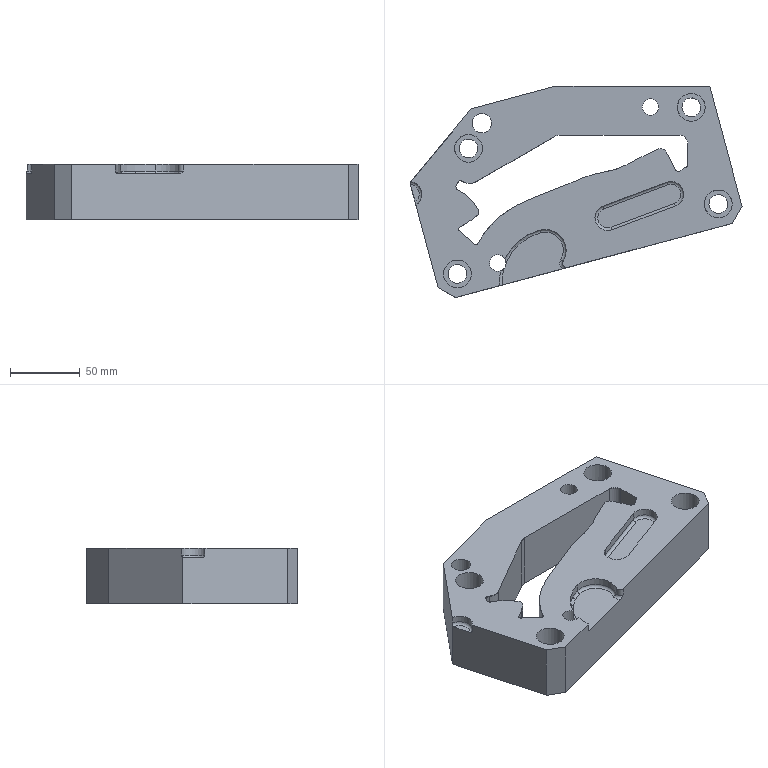Part | NX | features 23 2 | 1 solid | 112 faces | box 238.475 x 151.712 x 40 mm | volume 793319 mm3 | spline 46 | plane 35 | cylinder 24 | torus 7 | commonest cylinder face diameters 20 x6 13.5 x4 18.155 x3 4 x2 12.001 x2 16 x2